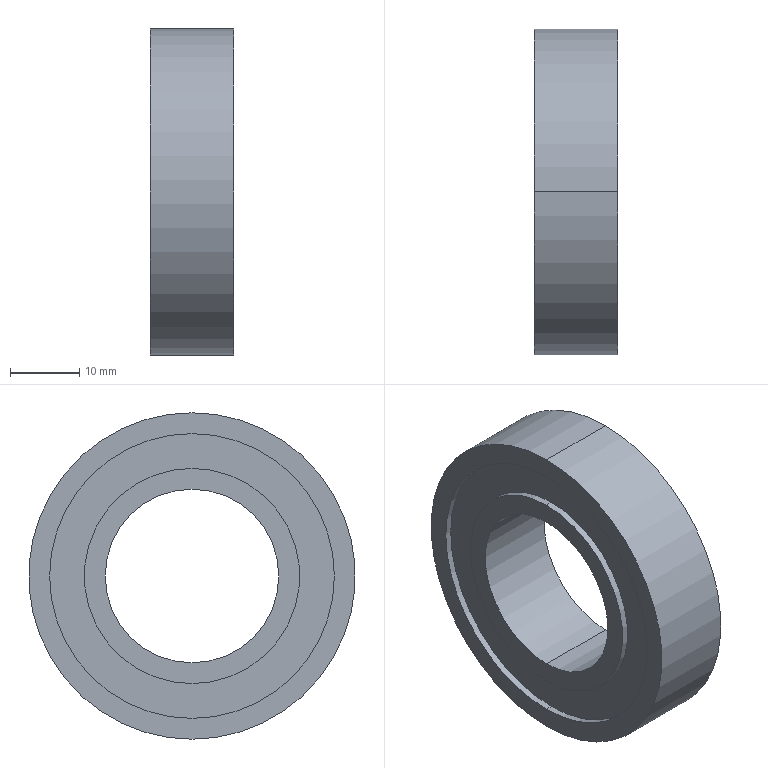Part | SolidWorks | features Revolution 1 | 1 solid | 18 faces | box 12 x 47 x 47 mm | volume 13798 mm3 | cylinder 12 | plane 6 | commonest cylinder face diameters 31 x4 41 x4 25 x2 47 x2
STEP:
#1=CARTESIAN_POINT('',(25.12,0.,-12.5));
#2=VERTEX_POINT('',#1);
#3=CARTESIAN_POINT('',(25.12,0.,12.5));
#4=VERTEX_POINT('',#3);
#5=CARTESIAN_POINT('',(25.12,0.,0.));
#6=DIRECTION('',(-1.,0.,0.));
#7=DIRECTION('',(0.,0.,1.));
#8=AXIS2_PLACEMENT_3D('',#5,#6,#7);
#9=CIRCLE('',#8,12.5);
#10=EDGE_CURVE('',#2,#4,#9,.T.);
#11=ORIENTED_EDGE('',*,*,#10,.F.);
#12=CARTESIAN_POINT('',(13.12,0.,-12.5));
#13=VERTEX_POINT('',#12);
#14=CARTESIAN_POINT('',(0.,0.,-12.5));
#15=DIRECTION('',(-1.,0.,0.));
#16=VECTOR('',#15,1000.);
#17=LINE('',#14,#16);
#18=EDGE_CURVE('',#2,#13,#17,.T.);
#19=ORIENTED_EDGE('',*,*,#18,.T.);
#20=CARTESIAN_POINT('',(13.12,0.,12.5));
#21=VERTEX_POINT('',#20);
#22=CARTESIAN_POINT('',(13.12,0.,0.));
#23=DIRECTION('',(-1.,0.,0.));
#24=DIRECTION('',(0.,0.,1.));
#25=AXIS2_PLACEMENT_3D('',#22,#23,#24);
#26=CIRCLE('',#25,12.5);
#27=EDGE_CURVE('',#13,#21,#26,.T.);
#28=ORIENTED_EDGE('',*,*,#27,.T.);
#29=CARTESIAN_POINT('',(0.,0.,12.5));
#30=DIRECTION('',(-1.,0.,0.));
#31=VECTOR('',#30,1000.);
#32=LINE('',#29,#31);
#33=EDGE_CURVE('',#4,#21,#32,.T.);
#34=ORIENTED_EDGE('',*,*,#33,.F.);
#35=EDGE_LOOP('',(#11,#19,#28,#34));
#36=FACE_OUTER_BOUND('',#35,.T.);
#37=CARTESIAN_POINT('',(0.,0.,0.));
#38=DIRECTION('',(-1.,0.,0.));
#39=DIRECTION('',(0.,0.,1.));
#40=AXIS2_PLACEMENT_3D('',#37,#38,#39);
#41=CYLINDRICAL_SURFACE('',#40,12.5);
#42=ADVANCED_FACE('',(#36),#41,.F.);
#43=CARTESIAN_POINT('',(25.12,0.,15.5));
#44=VERTEX_POINT('',#43);
#45=CARTESIAN_POINT('',(25.12,0.,-15.5));
#46=VERTEX_POINT('',#45);
#47=CARTESIAN_POINT('',(25.12,0.,0.));
#48=DIRECTION('',(-1.,0.,0.));
#49=DIRECTION('',(0.,0.,1.));
#50=AXIS2_PLACEMENT_3D('',#47,#48,#49);
#51=CIRCLE('',#50,15.5);
#52=EDGE_CURVE('',#44,#46,#51,.T.);
#53=ORIENTED_EDGE('',*,*,#52,.T.);
#54=CARTESIAN_POINT('',(24.12,0.,-15.5));
#55=VERTEX_POINT('',#54);
#56=CARTESIAN_POINT('',(0.,0.,-15.5));
#57=DIRECTION('',(-1.,0.,0.));
#58=VECTOR('',#57,1000.);
#59=LINE('',#56,#58);
#60=EDGE_CURVE('',#46,#55,#59,.T.);
#61=ORIENTED_EDGE('',*,*,#60,.T.);
#62=CARTESIAN_POINT('',(24.12,0.,15.5));
#63=VERTEX_POINT('',#62);
#64=CARTESIAN_POINT('',(24.12,0.,0.));
#65=DIRECTION('',(-1.,0.,0.));
#66=DIRECTION('',(0.,0.,1.));
#67=AXIS2_PLACEMENT_3D('',#64,#65,#66);
#68=CIRCLE('',#67,15.5);
#69=EDGE_CURVE('',#63,#55,#68,.T.);
#70=ORIENTED_EDGE('',*,*,#69,.F.);
#71=CARTESIAN_POINT('',(0.,0.,15.5));
#72=DIRECTION('',(-1.,0.,0.));
#73=VECTOR('',#72,1000.);
#74=LINE('',#71,#73);
#75=EDGE_CURVE('',#44,#63,#74,.T.);
#76=ORIENTED_EDGE('',*,*,#75,.F.);
#77=EDGE_LOOP('',(#53,#61,#70,#76));
#78=FACE_OUTER_BOUND('',#77,.T.);
#79=CARTESIAN_POINT('',(0.,0.,0.));
#80=DIRECTION('',(-1.,0.,0.));
#81=DIRECTION('',(0.,0.,1.));
#82=AXIS2_PLACEMENT_3D('',#79,#80,#81);
#83=CYLINDRICAL_SURFACE('',#82,15.5);
#84=ADVANCED_FACE('',(#78),#83,.T.);
#85=CARTESIAN_POINT('',(25.12,0.,-20.5));
#86=VERTEX_POINT('',#85);
#87=CARTESIAN_POINT('',(25.12,0.,20.5));
#88=VERTEX_POINT('',#87);
#89=CARTESIAN_POINT('',(25.12,0.,0.));
#90=DIRECTION('',(-1.,0.,0.));
#91=DIRECTION('',(0.,0.,1.));
#92=AXIS2_PLACEMENT_3D('',#89,#90,#91);
#93=CIRCLE('',#92,20.5);
#94=EDGE_CURVE('',#86,#88,#93,.T.);
#95=ORIENTED_EDGE('',*,*,#94,.F.);
#96=CARTESIAN_POINT('',(24.12,0.,-20.5));
#97=VERTEX_POINT('',#96);
#98=CARTESIAN_POINT('',(0.,0.,-20.5));
#99=DIRECTION('',(-1.,0.,0.));
#100=VECTOR('',#99,1000.);
#101=LINE('',#98,#100);
#102=EDGE_CURVE('',#86,#97,#101,.T.);
#103=ORIENTED_EDGE('',*,*,#102,.T.);
#104=CARTESIAN_POINT('',(24.12,0.,20.5));
#105=VERTEX_POINT('',#104);
#106=CARTESIAN_POINT('',(24.12,0.,0.));
#107=DIRECTION('',(-1.,0.,0.));
#108=DIRECTION('',(0.,0.,1.));
#109=AXIS2_PLACEMENT_3D('',#106,#107,#108);
#110=CIRCLE('',#109,20.5);
#111=EDGE_CURVE('',#97,#105,#110,.T.);
#112=ORIENTED_EDGE('',*,*,#111,.T.);
#113=CARTESIAN_POINT('',(0.,0.,20.5));
#114=DIRECTION('',(-1.,0.,0.));
#115=VECTOR('',#114,1000.);
#116=LINE('',#113,#115);
#117=EDGE_CURVE('',#88,#105,#116,.T.);
#118=ORIENTED_EDGE('',*,*,#117,.F.);
#119=EDGE_LOOP('',(#95,#103,#112,#118));
#120=FACE_OUTER_BOUND('',#119,.T.);
#121=CARTESIAN_POINT('',(0.,0.,0.));
#122=DIRECTION('',(-1.,0.,0.));
#123=DIRECTION('',(0.,0.,1.));
#124=AXIS2_PLACEMENT_3D('',#121,#122,#123);
#125=CYLINDRICAL_SURFACE('',#124,20.5);
#126=ADVANCED_FACE('',(#120),#125,.F.);
#127=CARTESIAN_POINT('',(25.12,0.,23.5));
#128=VERTEX_POINT('',#127);
#129=CARTESIAN_POINT('',(25.12,0.,-23.5));
#130=VERTEX_POINT('',#129);
#131=CARTESIAN_POINT('',(25.12,0.,0.));
#132=DIRECTION('',(-1.,0.,0.));
#133=DIRECTION('',(0.,0.,1.));
#134=AXIS2_PLACEMENT_3D('',#131,#132,#133);
#135=CIRCLE('',#134,23.5);
#136=EDGE_CURVE('',#128,#130,#135,.T.);
#137=ORIENTED_EDGE('',*,*,#136,.T.);
#138=CARTESIAN_POINT('',(13.12,0.,-23.5));
#139=VERTEX_POINT('',#138);
#140=CARTESIAN_POINT('',(0.,0.,-23.5));
#141=DIRECTION('',(-1.,0.,0.));
#142=VECTOR('',#141,1000.);
#143=LINE('',#140,#142);
#144=EDGE_CURVE('',#130,#139,#143,.T.);
#145=ORIENTED_EDGE('',*,*,#144,.T.);
#146=CARTESIAN_POINT('',(13.12,0.,23.5));
#147=VERTEX_POINT('',#146);
#148=CARTESIAN_POINT('',(13.12,0.,0.));
#149=DIRECTION('',(-1.,0.,0.));
#150=DIRECTION('',(0.,0.,1.));
#151=AXIS2_PLACEMENT_3D('',#148,#149,#150);
#152=CIRCLE('',#151,23.5);
#153=EDGE_CURVE('',#147,#139,#152,.T.);
#154=ORIENTED_EDGE('',*,*,#153,.F.);
#155=CARTESIAN_POINT('',(0.,0.,23.5));
#156=DIRECTION('',(-1.,0.,0.));
#157=VECTOR('',#156,1000.);
#158=LINE('',#155,#157);
#159=EDGE_CURVE('',#128,#147,#158,.T.);
#160=ORIENTED_EDGE('',*,*,#159,.F.);
#161=EDGE_LOOP('',(#137,#145,#154,#160));
#162=FACE_OUTER_BOUND('',#161,.T.);
#163=CARTESIAN_POINT('',(0.,0.,0.));
#164=DIRECTION('',(-1.,0.,0.));
#165=DIRECTION('',(0.,0.,1.));
#166=AXIS2_PLACEMENT_3D('',#163,#164,#165);
#167=CYLINDRICAL_SURFACE('',#166,23.5);
#168=ADVANCED_FACE('',(#162),#167,.T.);
#169=CARTESIAN_POINT('',(14.12,0.,-20.5));
#170=VERTEX_POINT('',#169);
#171=CARTESIAN_POINT('',(14.12,0.,20.5));
#172=VERTEX_POINT('',#171);
#173=CARTESIAN_POINT('',(14.12,0.,0.));
#174=DIRECTION('',(-1.,0.,0.));
#175=DIRECTION('',(0.,0.,1.));
#176=AXIS2_PLACEMENT_3D('',#173,#174,#175);
#177=CIRCLE('',#176,20.5);
#178=EDGE_CURVE('',#170,#172,#177,.T.);
#179=ORIENTED_EDGE('',*,*,#178,.F.);
#180=CARTESIAN_POINT('',(13.12,0.,-20.5));
#181=VERTEX_POINT('',#180);
#182=CARTESIAN_POINT('',(0.,0.,-20.5));
#183=DIRECTION('',(-1.,0.,0.));
#184=VECTOR('',#183,1000.);
#185=LINE('',#182,#184);
#186=EDGE_CURVE('',#170,#181,#185,.T.);
#187=ORIENTED_EDGE('',*,*,#186,.T.);
#188=CARTESIAN_POINT('',(13.12,0.,20.5));
#189=VERTEX_POINT('',#188);
#190=CARTESIAN_POINT('',(13.12,0.,0.));
#191=DIRECTION('',(-1.,0.,0.));
#192=DIRECTION('',(0.,0.,1.));
#193=AXIS2_PLACEMENT_3D('',#190,#191,#192);
#194=CIRCLE('',#193,20.5);
#195=EDGE_CURVE('',#181,#189,#194,.T.);
#196=ORIENTED_EDGE('',*,*,#195,.T.);
#197=CARTESIAN_POINT('',(0.,0.,20.5));
#198=DIRECTION('',(-1.,0.,0.));
#199=VECTOR('',#198,1000.);
#200=LINE('',#197,#199);
#201=EDGE_CURVE('',#172,#189,#200,.T.);
#202=ORIENTED_EDGE('',*,*,#201,.F.);
#203=EDGE_LOOP('',(#179,#187,#196,#202));
#204=FACE_OUTER_BOUND('',#203,.T.);
#205=CARTESIAN_POINT('',(0.,0.,0.));
#206=DIRECTION('',(-1.,0.,0.));
#207=DIRECTION('',(0.,0.,1.));
#208=AXIS2_PLACEMENT_3D('',#205,#206,#207);
#209=CYLINDRICAL_SURFACE('',#208,20.5);
#210=ADVANCED_FACE('',(#204),#209,.F.);
#211=CARTESIAN_POINT('',(14.12,0.,15.5));
#212=VERTEX_POINT('',#211);
#213=CARTESIAN_POINT('',(14.12,0.,-15.5));
#214=VERTEX_POINT('',#213);
#215=CARTESIAN_POINT('',(14.12,0.,0.));
#216=DIRECTION('',(-1.,0.,0.));
#217=DIRECTION('',(0.,0.,1.));
#218=AXIS2_PLACEMENT_3D('',#215,#216,#217);
#219=CIRCLE('',#218,15.5);
#220=EDGE_CURVE('',#212,#214,#219,.T.);
#221=ORIENTED_EDGE('',*,*,#220,.T.);
#222=CARTESIAN_POINT('',(13.12,0.,-15.5));
#223=VERTEX_POINT('',#222);
#224=CARTESIAN_POINT('',(0.,0.,-15.5));
#225=DIRECTION('',(-1.,0.,0.));
#226=VECTOR('',#225,1000.);
#227=LINE('',#224,#226);
#228=EDGE_CURVE('',#214,#223,#227,.T.);
#229=ORIENTED_EDGE('',*,*,#228,.T.);
#230=CARTESIAN_POINT('',(13.12,0.,15.5));
#231=VERTEX_POINT('',#230);
#232=CARTESIAN_POINT('',(13.12,0.,0.));
#233=DIRECTION('',(-1.,0.,0.));
#234=DIRECTION('',(0.,0.,1.));
#235=AXIS2_PLACEMENT_3D('',#232,#233,#234);
#236=CIRCLE('',#235,15.5);
#237=EDGE_CURVE('',#231,#223,#236,.T.);
#238=ORIENTED_EDGE('',*,*,#237,.F.);
#239=CARTESIAN_POINT('',(0.,0.,15.5));
#240=DIRECTION('',(-1.,0.,0.));
#241=VECTOR('',#240,1000.);
#242=LINE('',#239,#241);
#243=EDGE_CURVE('',#212,#231,#242,.T.);
#244=ORIENTED_EDGE('',*,*,#243,.F.);
#245=EDGE_LOOP('',(#221,#229,#238,#244));
#246=FACE_OUTER_BOUND('',#245,.T.);
#247=CARTESIAN_POINT('',(0.,0.,0.));
#248=DIRECTION('',(-1.,0.,0.));
#249=DIRECTION('',(0.,0.,1.));
#250=AXIS2_PLACEMENT_3D('',#247,#248,#249);
#251=CYLINDRICAL_SURFACE('',#250,15.5);
#252=ADVANCED_FACE('',(#246),#251,.T.);
#253=CARTESIAN_POINT('',(13.12,0.,0.));
#254=DIRECTION('',(-1.,0.,0.));
#255=DIRECTION('',(0.,0.,1.));
#256=AXIS2_PLACEMENT_3D('',#253,#254,#255);
#257=CIRCLE('',#256,12.5);
#258=EDGE_CURVE('',#21,#13,#257,.T.);
#259=ORIENTED_EDGE('',*,*,#258,.F.);
#260=ORIENTED_EDGE('',*,*,#27,.F.);
#261=EDGE_LOOP('',(#259,#260));
#262=FACE_BOUND('',#261,.T.);
#263=ORIENTED_EDGE('',*,*,#237,.T.);
#264=CARTESIAN_POINT('',(13.12,0.,0.));
#265=DIRECTION('',(-1.,0.,0.));
#266=DIRECTION('',(0.,0.,1.));
#267=AXIS2_PLACEMENT_3D('',#264,#265,#266);
#268=CIRCLE('',#267,15.5);
#269=EDGE_CURVE('',#223,#231,#268,.T.);
#270=ORIENTED_EDGE('',*,*,#269,.T.);
#271=EDGE_LOOP('',(#263,#270));
#272=FACE_OUTER_BOUND('',#271,.T.);
#273=CARTESIAN_POINT('',(13.12,12.5,0.));
#274=DIRECTION('',(1.,0.,0.));
#275=DIRECTION('',(0.,0.,-1.));
#276=AXIS2_PLACEMENT_3D('',#273,#274,#275);
#277=PLANE('',#276);
#278=ADVANCED_FACE('',(#262,#272),#277,.F.);
#279=ORIENTED_EDGE('',*,*,#228,.F.);
#280=CARTESIAN_POINT('',(14.12,0.,0.));
#281=DIRECTION('',(-1.,0.,0.));
#282=DIRECTION('',(0.,0.,1.));
#283=AXIS2_PLACEMENT_3D('',#280,#281,#282);
#284=CIRCLE('',#283,15.5);
#285=EDGE_CURVE('',#214,#212,#284,.T.);
#286=ORIENTED_EDGE('',*,*,#285,.T.);
#287=ORIENTED_EDGE('',*,*,#243,.T.);
#288=ORIENTED_EDGE('',*,*,#269,.F.);
#289=EDGE_LOOP('',(#279,#286,#287,#288));
#290=FACE_OUTER_BOUND('',#289,.T.);
#291=CARTESIAN_POINT('',(0.,0.,0.));
#292=DIRECTION('',(-1.,0.,0.));
#293=DIRECTION('',(0.,0.,1.));
#294=AXIS2_PLACEMENT_3D('',#291,#292,#293);
#295=CYLINDRICAL_SURFACE('',#294,15.5);
#296=ADVANCED_FACE('',(#290),#295,.T.);
#297=ORIENTED_EDGE('',*,*,#220,.F.);
#298=ORIENTED_EDGE('',*,*,#285,.F.);
#299=EDGE_LOOP('',(#297,#298));
#300=FACE_BOUND('',#299,.T.);
#301=CARTESIAN_POINT('',(14.12,0.,0.));
#302=DIRECTION('',(-1.,0.,0.));
#303=DIRECTION('',(0.,0.,1.));
#304=AXIS2_PLACEMENT_3D('',#301,#302,#303);
#305=CIRCLE('',#304,20.5);
#306=EDGE_CURVE('',#172,#170,#305,.T.);
#307=ORIENTED_EDGE('',*,*,#306,.T.);
#308=ORIENTED_EDGE('',*,*,#178,.T.);
#309=EDGE_LOOP('',(#307,#308));
#310=FACE_OUTER_BOUND('',#309,.T.);
#311=CARTESIAN_POINT('',(14.12,15.5,0.));
#312=DIRECTION('',(1.,0.,0.));
#313=DIRECTION('',(0.,0.,-1.));
#314=AXIS2_PLACEMENT_3D('',#311,#312,#313);
#315=PLANE('',#314);
#316=ADVANCED_FACE('',(#300,#310),#315,.F.);
#317=ORIENTED_EDGE('',*,*,#186,.F.);
#318=ORIENTED_EDGE('',*,*,#306,.F.);
#319=ORIENTED_EDGE('',*,*,#201,.T.);
#320=CARTESIAN_POINT('',(13.12,0.,0.));
#321=DIRECTION('',(-1.,0.,0.));
#322=DIRECTION('',(0.,0.,1.));
#323=AXIS2_PLACEMENT_3D('',#320,#321,#322);
#324=CIRCLE('',#323,20.5);
#325=EDGE_CURVE('',#189,#181,#324,.T.);
#326=ORIENTED_EDGE('',*,*,#325,.T.);
#327=EDGE_LOOP('',(#317,#318,#319,#326));
#328=FACE_OUTER_BOUND('',#327,.T.);
#329=CARTESIAN_POINT('',(0.,0.,0.));
#330=DIRECTION('',(-1.,0.,0.));
#331=DIRECTION('',(0.,0.,1.));
#332=AXIS2_PLACEMENT_3D('',#329,#330,#331);
#333=CYLINDRICAL_SURFACE('',#332,20.5);
#334=ADVANCED_FACE('',(#328),#333,.F.);
#335=ORIENTED_EDGE('',*,*,#325,.F.);
#336=ORIENTED_EDGE('',*,*,#195,.F.);
#337=EDGE_LOOP('',(#335,#336));
#338=FACE_BOUND('',#337,.T.);
#339=ORIENTED_EDGE('',*,*,#153,.T.);
#340=CARTESIAN_POINT('',(13.12,0.,0.));
#341=DIRECTION('',(-1.,0.,0.));
#342=DIRECTION('',(0.,0.,1.));
#343=AXIS2_PLACEMENT_3D('',#340,#341,#342);
#344=CIRCLE('',#343,23.5);
#345=EDGE_CURVE('',#139,#147,#344,.T.);
#346=ORIENTED_EDGE('',*,*,#345,.T.);
#347=EDGE_LOOP('',(#339,#346));
#348=FACE_OUTER_BOUND('',#347,.T.);
#349=CARTESIAN_POINT('',(13.12,20.5,0.));
#350=DIRECTION('',(1.,0.,0.));
#351=DIRECTION('',(0.,0.,-1.));
#352=AXIS2_PLACEMENT_3D('',#349,#350,#351);
#353=PLANE('',#352);
#354=ADVANCED_FACE('',(#338,#348),#353,.F.);
#355=ORIENTED_EDGE('',*,*,#144,.F.);
#356=CARTESIAN_POINT('',(25.12,0.,0.));
#357=DIRECTION('',(-1.,0.,0.));
#358=DIRECTION('',(0.,0.,1.));
#359=AXIS2_PLACEMENT_3D('',#356,#357,#358);
#360=CIRCLE('',#359,23.5);
#361=EDGE_CURVE('',#130,#128,#360,.T.);
#362=ORIENTED_EDGE('',*,*,#361,.T.);
#363=ORIENTED_EDGE('',*,*,#159,.T.);
#364=ORIENTED_EDGE('',*,*,#345,.F.);
#365=EDGE_LOOP('',(#355,#362,#363,#364));
#366=FACE_OUTER_BOUND('',#365,.T.);
#367=CARTESIAN_POINT('',(0.,0.,0.));
#368=DIRECTION('',(-1.,0.,0.));
#369=DIRECTION('',(0.,0.,1.));
#370=AXIS2_PLACEMENT_3D('',#367,#368,#369);
#371=CYLINDRICAL_SURFACE('',#370,23.5);
#372=ADVANCED_FACE('',(#366),#371,.T.);
#373=ORIENTED_EDGE('',*,*,#136,.F.);
#374=ORIENTED_EDGE('',*,*,#361,.F.);
#375=EDGE_LOOP('',(#373,#374));
#376=FACE_OUTER_BOUND('',#375,.T.);
#377=CARTESIAN_POINT('',(25.12,0.,0.));
#378=DIRECTION('',(-1.,0.,0.));
#379=DIRECTION('',(0.,0.,1.));
#380=AXIS2_PLACEMENT_3D('',#377,#378,#379);
#381=CIRCLE('',#380,20.5);
#382=EDGE_CURVE('',#88,#86,#381,.T.);
#383=ORIENTED_EDGE('',*,*,#382,.T.);
#384=ORIENTED_EDGE('',*,*,#94,.T.);
#385=EDGE_LOOP('',(#383,#384));
#386=FACE_BOUND('',#385,.T.);
#387=CARTESIAN_POINT('',(25.12,20.5,0.));
#388=DIRECTION('',(-1.,0.,0.));
#389=DIRECTION('',(0.,0.,1.));
#390=AXIS2_PLACEMENT_3D('',#387,#388,#389);
#391=PLANE('',#390);
#392=ADVANCED_FACE('',(#376,#386),#391,.F.);
#393=ORIENTED_EDGE('',*,*,#102,.F.);
#394=ORIENTED_EDGE('',*,*,#382,.F.);
#395=ORIENTED_EDGE('',*,*,#117,.T.);
#396=CARTESIAN_POINT('',(24.12,0.,0.));
#397=DIRECTION('',(-1.,0.,0.));
#398=DIRECTION('',(0.,0.,1.));
#399=AXIS2_PLACEMENT_3D('',#396,#397,#398);
#400=CIRCLE('',#399,20.5);
#401=EDGE_CURVE('',#105,#97,#400,.T.);
#402=ORIENTED_EDGE('',*,*,#401,.T.);
#403=EDGE_LOOP('',(#393,#394,#395,#402));
#404=FACE_OUTER_BOUND('',#403,.T.);
#405=CARTESIAN_POINT('',(0.,0.,0.));
#406=DIRECTION('',(-1.,0.,0.));
#407=DIRECTION('',(0.,0.,1.));
#408=AXIS2_PLACEMENT_3D('',#405,#406,#407);
#409=CYLINDRICAL_SURFACE('',#408,20.5);
#410=ADVANCED_FACE('',(#404),#409,.F.);
#411=ORIENTED_EDGE('',*,*,#401,.F.);
#412=ORIENTED_EDGE('',*,*,#111,.F.);
#413=EDGE_LOOP('',(#411,#412));
#414=FACE_OUTER_BOUND('',#413,.T.);
#415=ORIENTED_EDGE('',*,*,#69,.T.);
#416=CARTESIAN_POINT('',(24.12,0.,0.));
#417=DIRECTION('',(-1.,0.,0.));
#418=DIRECTION('',(0.,0.,1.));
#419=AXIS2_PLACEMENT_3D('',#416,#417,#418);
#420=CIRCLE('',#419,15.5);
#421=EDGE_CURVE('',#55,#63,#420,.T.);
#422=ORIENTED_EDGE('',*,*,#421,.T.);
#423=EDGE_LOOP('',(#415,#422));
#424=FACE_BOUND('',#423,.T.);
#425=CARTESIAN_POINT('',(24.12,15.5,0.));
#426=DIRECTION('',(-1.,0.,0.));
#427=DIRECTION('',(0.,0.,1.));
#428=AXIS2_PLACEMENT_3D('',#425,#426,#427);
#429=PLANE('',#428);
#430=ADVANCED_FACE('',(#414,#424),#429,.F.);
#431=ORIENTED_EDGE('',*,*,#60,.F.);
#432=CARTESIAN_POINT('',(25.12,0.,0.));
#433=DIRECTION('',(-1.,0.,0.));
#434=DIRECTION('',(0.,0.,1.));
#435=AXIS2_PLACEMENT_3D('',#432,#433,#434);
#436=CIRCLE('',#435,15.5);
#437=EDGE_CURVE('',#46,#44,#436,.T.);
#438=ORIENTED_EDGE('',*,*,#437,.T.);
#439=ORIENTED_EDGE('',*,*,#75,.T.);
#440=ORIENTED_EDGE('',*,*,#421,.F.);
#441=EDGE_LOOP('',(#431,#438,#439,#440));
#442=FACE_OUTER_BOUND('',#441,.T.);
#443=CARTESIAN_POINT('',(0.,0.,0.));
#444=DIRECTION('',(-1.,0.,0.));
#445=DIRECTION('',(0.,0.,1.));
#446=AXIS2_PLACEMENT_3D('',#443,#444,#445);
#447=CYLINDRICAL_SURFACE('',#446,15.5);
#448=ADVANCED_FACE('',(#442),#447,.T.);
#449=ORIENTED_EDGE('',*,*,#52,.F.);
#450=ORIENTED_EDGE('',*,*,#437,.F.);
#451=EDGE_LOOP('',(#449,#450));
#452=FACE_OUTER_BOUND('',#451,.T.);
#453=CARTESIAN_POINT('',(25.12,0.,0.));
#454=DIRECTION('',(-1.,0.,0.));
#455=DIRECTION('',(0.,0.,1.));
#456=AXIS2_PLACEMENT_3D('',#453,#454,#455);
#457=CIRCLE('',#456,12.5);
#458=EDGE_CURVE('',#4,#2,#457,.T.);
#459=ORIENTED_EDGE('',*,*,#458,.T.);
#460=ORIENTED_EDGE('',*,*,#10,.T.);
#461=EDGE_LOOP('',(#459,#460));
#462=FACE_BOUND('',#461,.T.);
#463=CARTESIAN_POINT('',(25.12,12.5,0.));
#464=DIRECTION('',(-1.,0.,0.));
#465=DIRECTION('',(0.,0.,1.));
#466=AXIS2_PLACEMENT_3D('',#463,#464,#465);
#467=PLANE('',#466);
#468=ADVANCED_FACE('',(#452,#462),#467,.F.);
#469=ORIENTED_EDGE('',*,*,#18,.F.);
#470=ORIENTED_EDGE('',*,*,#458,.F.);
#471=ORIENTED_EDGE('',*,*,#33,.T.);
#472=ORIENTED_EDGE('',*,*,#258,.T.);
#473=EDGE_LOOP('',(#469,#470,#471,#472));
#474=FACE_OUTER_BOUND('',#473,.T.);
#475=CARTESIAN_POINT('',(0.,0.,0.));
#476=DIRECTION('',(-1.,0.,0.));
#477=DIRECTION('',(0.,0.,1.));
#478=AXIS2_PLACEMENT_3D('',#475,#476,#477);
#479=CYLINDRICAL_SURFACE('',#478,12.5);
#480=ADVANCED_FACE('',(#474),#479,.F.);
#481=CLOSED_SHELL('',(#42,#84,#126,#168,#210,#252,#278,#296,#316,#334,#354,#372,#392,#410,#430,#448,#468,#480));
#482=MANIFOLD_SOLID_BREP('',#481);
#483=CARTESIAN_POINT('',(0.,0.,0.));
#484=DIRECTION('',(0.,0.,1.));
#485=DIRECTION('',(1.,0.,0.));
#486=AXIS2_PLACEMENT_3D('',#483,#484,#485);
#487=(LENGTH_UNIT()NAMED_UNIT(*)SI_UNIT(.MILLI.,.METRE.));
#488=UNCERTAINTY_MEASURE_WITH_UNIT(LENGTH_MEASURE(0.00001),#487,'','');
#489=(NAMED_UNIT(*)PLANE_ANGLE_UNIT()SI_UNIT($,.RADIAN.));
#490=(NAMED_UNIT(*)SI_UNIT($,.STERADIAN.)SOLID_ANGLE_UNIT());
#491=(GEOMETRIC_REPRESENTATION_CONTEXT(3)GLOBAL_UNCERTAINTY_ASSIGNED_CONTEXT((#488))GLOBAL_UNIT_ASSIGNED_CONTEXT((#487,#489,#490))REPRESENTATION_CONTEXT('',''));
#492=ADVANCED_BREP_SHAPE_REPRESENTATION('',(#482,#486),#491);